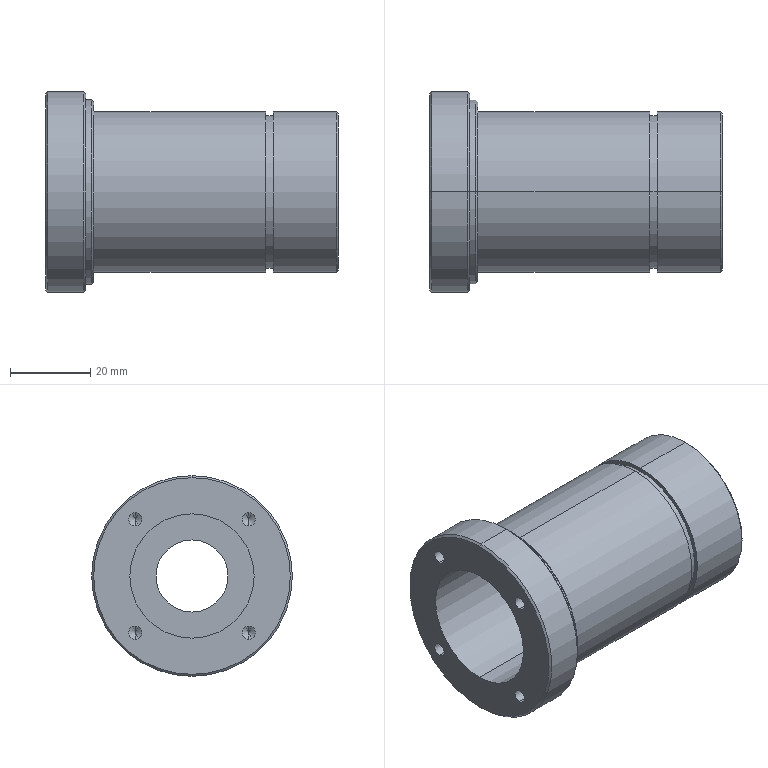Part | STEP file | PN_0039 Shaft_Default | 1 solid | 61 faces | box 73 x 50 x 50 mm | volume 53647 mm3 | cylinder 30 | cone 24 | plane 7 | commonest cylinder face diameters 3.3 x8 4.2 x8 40 x4 18 x2 31 x2 38 x2